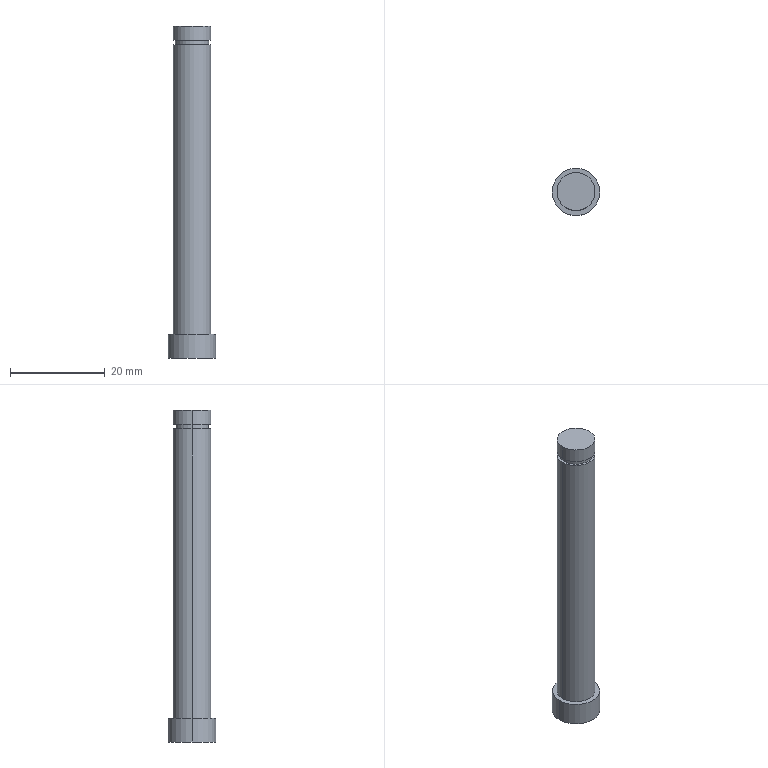Part | SolidWorks | features BaseBody 1 | 1 solid | 13 faces | box 10 x 10 x 70 mm | volume 3648 mm3 | cylinder 8 | plane 5 | commonest cylinder face diameters 8 x4 7 x2 10 x2
STEP:
#1=CARTESIAN_POINT('',(-4.,0.,67.));
#2=VERTEX_POINT('',#1);
#3=CARTESIAN_POINT('',(4.,0.,67.));
#4=VERTEX_POINT('',#3);
#5=CARTESIAN_POINT('',(0.,0.,67.));
#6=DIRECTION('',(0.,0.,-1.));
#7=DIRECTION('',(1.,0.,0.));
#8=AXIS2_PLACEMENT_3D('',#5,#6,#7);
#9=CIRCLE('',#8,4.);
#10=EDGE_CURVE('',#2,#4,#9,.T.);
#11=ORIENTED_EDGE('',*,*,#10,.F.);
#12=CARTESIAN_POINT('',(-4.,0.,70.));
#13=VERTEX_POINT('',#12);
#14=CARTESIAN_POINT('',(-4.,0.,5.));
#15=DIRECTION('',(0.,0.,1.));
#16=VECTOR('',#15,1000.);
#17=LINE('',#14,#16);
#18=EDGE_CURVE('',#2,#13,#17,.T.);
#19=ORIENTED_EDGE('',*,*,#18,.T.);
#20=CARTESIAN_POINT('',(4.,0.,70.));
#21=VERTEX_POINT('',#20);
#22=CARTESIAN_POINT('',(0.,0.,70.));
#23=DIRECTION('',(0.,0.,1.));
#24=DIRECTION('',(1.,0.,0.));
#25=AXIS2_PLACEMENT_3D('',#22,#23,#24);
#26=CIRCLE('',#25,4.);
#27=EDGE_CURVE('',#21,#13,#26,.T.);
#28=ORIENTED_EDGE('',*,*,#27,.F.);
#29=CARTESIAN_POINT('',(4.,0.,5.));
#30=DIRECTION('',(0.,0.,1.));
#31=VECTOR('',#30,1000.);
#32=LINE('',#29,#31);
#33=EDGE_CURVE('',#4,#21,#32,.T.);
#34=ORIENTED_EDGE('',*,*,#33,.F.);
#35=EDGE_LOOP('',(#11,#19,#28,#34));
#36=FACE_OUTER_BOUND('',#35,.T.);
#37=CARTESIAN_POINT('',(0.,0.,5.));
#38=DIRECTION('',(0.,0.,1.));
#39=DIRECTION('',(1.,0.,0.));
#40=AXIS2_PLACEMENT_3D('',#37,#38,#39);
#41=CYLINDRICAL_SURFACE('',#40,4.);
#42=ADVANCED_FACE('',(#36),#41,.T.);
#43=CARTESIAN_POINT('',(3.5,0.,66.));
#44=VERTEX_POINT('',#43);
#45=CARTESIAN_POINT('',(-3.5,0.,66.));
#46=VERTEX_POINT('',#45);
#47=CARTESIAN_POINT('',(0.,0.,66.));
#48=DIRECTION('',(0.,0.,1.));
#49=DIRECTION('',(1.,0.,0.));
#50=AXIS2_PLACEMENT_3D('',#47,#48,#49);
#51=CIRCLE('',#50,3.5);
#52=EDGE_CURVE('',#44,#46,#51,.T.);
#53=ORIENTED_EDGE('',*,*,#52,.T.);
#54=CARTESIAN_POINT('',(-3.5,0.,67.));
#55=VERTEX_POINT('',#54);
#56=CARTESIAN_POINT('',(-3.5,0.,66.));
#57=DIRECTION('',(0.,0.,1.));
#58=VECTOR('',#57,1000.);
#59=LINE('',#56,#58);
#60=EDGE_CURVE('',#46,#55,#59,.T.);
#61=ORIENTED_EDGE('',*,*,#60,.T.);
#62=CARTESIAN_POINT('',(3.5,0.,67.));
#63=VERTEX_POINT('',#62);
#64=CARTESIAN_POINT('',(0.,0.,67.));
#65=DIRECTION('',(0.,0.,1.));
#66=DIRECTION('',(1.,0.,0.));
#67=AXIS2_PLACEMENT_3D('',#64,#65,#66);
#68=CIRCLE('',#67,3.5);
#69=EDGE_CURVE('',#63,#55,#68,.T.);
#70=ORIENTED_EDGE('',*,*,#69,.F.);
#71=CARTESIAN_POINT('',(3.5,0.,66.));
#72=DIRECTION('',(0.,0.,1.));
#73=VECTOR('',#72,1000.);
#74=LINE('',#71,#73);
#75=EDGE_CURVE('',#44,#63,#74,.T.);
#76=ORIENTED_EDGE('',*,*,#75,.F.);
#77=EDGE_LOOP('',(#53,#61,#70,#76));
#78=FACE_OUTER_BOUND('',#77,.T.);
#79=CARTESIAN_POINT('',(0.,0.,66.));
#80=DIRECTION('',(0.,0.,1.));
#81=DIRECTION('',(1.,0.,0.));
#82=AXIS2_PLACEMENT_3D('',#79,#80,#81);
#83=CYLINDRICAL_SURFACE('',#82,3.5);
#84=ADVANCED_FACE('',(#78),#83,.T.);
#85=CARTESIAN_POINT('',(5.,0.,5.));
#86=VERTEX_POINT('',#85);
#87=CARTESIAN_POINT('',(-5.,0.,5.));
#88=VERTEX_POINT('',#87);
#89=CARTESIAN_POINT('',(0.,0.,5.));
#90=DIRECTION('',(0.,0.,1.));
#91=DIRECTION('',(1.,0.,0.));
#92=AXIS2_PLACEMENT_3D('',#89,#90,#91);
#93=CIRCLE('',#92,5.);
#94=EDGE_CURVE('',#86,#88,#93,.T.);
#95=ORIENTED_EDGE('',*,*,#94,.F.);
#96=CARTESIAN_POINT('',(5.,0.,0.));
#97=VERTEX_POINT('',#96);
#98=CARTESIAN_POINT('',(5.,0.,70.));
#99=DIRECTION('',(0.,0.,-1.));
#100=VECTOR('',#99,1000.);
#101=LINE('',#98,#100);
#102=EDGE_CURVE('',#86,#97,#101,.T.);
#103=ORIENTED_EDGE('',*,*,#102,.T.);
#104=CARTESIAN_POINT('',(-5.,0.,0.));
#105=VERTEX_POINT('',#104);
#106=CARTESIAN_POINT('',(0.,0.,0.));
#107=DIRECTION('',(0.,0.,1.));
#108=DIRECTION('',(1.,0.,0.));
#109=AXIS2_PLACEMENT_3D('',#106,#107,#108);
#110=CIRCLE('',#109,5.);
#111=EDGE_CURVE('',#97,#105,#110,.T.);
#112=ORIENTED_EDGE('',*,*,#111,.T.);
#113=CARTESIAN_POINT('',(-5.,0.,70.));
#114=DIRECTION('',(0.,0.,-1.));
#115=VECTOR('',#114,1000.);
#116=LINE('',#113,#115);
#117=EDGE_CURVE('',#88,#105,#116,.T.);
#118=ORIENTED_EDGE('',*,*,#117,.F.);
#119=EDGE_LOOP('',(#95,#103,#112,#118));
#120=FACE_OUTER_BOUND('',#119,.T.);
#121=CARTESIAN_POINT('',(0.,0.,70.));
#122=DIRECTION('',(0.,0.,-1.));
#123=DIRECTION('',(-1.,0.,0.));
#124=AXIS2_PLACEMENT_3D('',#121,#122,#123);
#125=CYLINDRICAL_SURFACE('',#124,5.);
#126=ADVANCED_FACE('',(#120),#125,.T.);
#127=CARTESIAN_POINT('',(4.,0.,5.));
#128=VERTEX_POINT('',#127);
#129=CARTESIAN_POINT('',(-4.,0.,5.));
#130=VERTEX_POINT('',#129);
#131=CARTESIAN_POINT('',(0.,0.,5.));
#132=DIRECTION('',(0.,0.,1.));
#133=DIRECTION('',(1.,0.,0.));
#134=AXIS2_PLACEMENT_3D('',#131,#132,#133);
#135=CIRCLE('',#134,4.);
#136=EDGE_CURVE('',#128,#130,#135,.T.);
#137=ORIENTED_EDGE('',*,*,#136,.T.);
#138=CARTESIAN_POINT('',(-4.,0.,66.));
#139=VERTEX_POINT('',#138);
#140=CARTESIAN_POINT('',(-4.,0.,5.));
#141=DIRECTION('',(0.,0.,1.));
#142=VECTOR('',#141,1000.);
#143=LINE('',#140,#142);
#144=EDGE_CURVE('',#130,#139,#143,.T.);
#145=ORIENTED_EDGE('',*,*,#144,.T.);
#146=CARTESIAN_POINT('',(4.,0.,66.));
#147=VERTEX_POINT('',#146);
#148=CARTESIAN_POINT('',(0.,0.,66.));
#149=DIRECTION('',(0.,0.,-1.));
#150=DIRECTION('',(1.,0.,0.));
#151=AXIS2_PLACEMENT_3D('',#148,#149,#150);
#152=CIRCLE('',#151,4.);
#153=EDGE_CURVE('',#139,#147,#152,.T.);
#154=ORIENTED_EDGE('',*,*,#153,.T.);
#155=CARTESIAN_POINT('',(4.,0.,5.));
#156=DIRECTION('',(0.,0.,1.));
#157=VECTOR('',#156,1000.);
#158=LINE('',#155,#157);
#159=EDGE_CURVE('',#128,#147,#158,.T.);
#160=ORIENTED_EDGE('',*,*,#159,.F.);
#161=EDGE_LOOP('',(#137,#145,#154,#160));
#162=FACE_OUTER_BOUND('',#161,.T.);
#163=CARTESIAN_POINT('',(0.,0.,5.));
#164=DIRECTION('',(0.,0.,1.));
#165=DIRECTION('',(1.,0.,0.));
#166=AXIS2_PLACEMENT_3D('',#163,#164,#165);
#167=CYLINDRICAL_SURFACE('',#166,4.);
#168=ADVANCED_FACE('',(#162),#167,.T.);
#169=ORIENTED_EDGE('',*,*,#27,.T.);
#170=CARTESIAN_POINT('',(0.,0.,70.));
#171=DIRECTION('',(0.,0.,1.));
#172=DIRECTION('',(1.,0.,0.));
#173=AXIS2_PLACEMENT_3D('',#170,#171,#172);
#174=CIRCLE('',#173,4.);
#175=EDGE_CURVE('',#13,#21,#174,.T.);
#176=ORIENTED_EDGE('',*,*,#175,.T.);
#177=EDGE_LOOP('',(#169,#176));
#178=FACE_OUTER_BOUND('',#177,.T.);
#179=CARTESIAN_POINT('',(0.,0.,70.));
#180=DIRECTION('',(0.,0.,1.));
#181=DIRECTION('',(1.,0.,0.));
#182=AXIS2_PLACEMENT_3D('',#179,#180,#181);
#183=PLANE('',#182);
#184=ADVANCED_FACE('',(#178),#183,.T.);
#185=ORIENTED_EDGE('',*,*,#69,.T.);
#186=CARTESIAN_POINT('',(0.,0.,67.));
#187=DIRECTION('',(0.,0.,1.));
#188=DIRECTION('',(1.,0.,0.));
#189=AXIS2_PLACEMENT_3D('',#186,#187,#188);
#190=CIRCLE('',#189,3.5);
#191=EDGE_CURVE('',#55,#63,#190,.T.);
#192=ORIENTED_EDGE('',*,*,#191,.T.);
#193=EDGE_LOOP('',(#185,#192));
#194=FACE_BOUND('',#193,.T.);
#195=CARTESIAN_POINT('',(0.,0.,67.));
#196=DIRECTION('',(0.,0.,-1.));
#197=DIRECTION('',(1.,0.,0.));
#198=AXIS2_PLACEMENT_3D('',#195,#196,#197);
#199=CIRCLE('',#198,4.);
#200=EDGE_CURVE('',#4,#2,#199,.T.);
#201=ORIENTED_EDGE('',*,*,#200,.T.);
#202=ORIENTED_EDGE('',*,*,#10,.T.);
#203=EDGE_LOOP('',(#201,#202));
#204=FACE_OUTER_BOUND('',#203,.T.);
#205=CARTESIAN_POINT('',(0.,0.,67.));
#206=DIRECTION('',(0.,0.,1.));
#207=DIRECTION('',(1.,0.,0.));
#208=AXIS2_PLACEMENT_3D('',#205,#206,#207);
#209=PLANE('',#208);
#210=ADVANCED_FACE('',(#194,#204),#209,.F.);
#211=ORIENTED_EDGE('',*,*,#52,.F.);
#212=CARTESIAN_POINT('',(0.,0.,66.));
#213=DIRECTION('',(0.,0.,1.));
#214=DIRECTION('',(1.,0.,0.));
#215=AXIS2_PLACEMENT_3D('',#212,#213,#214);
#216=CIRCLE('',#215,3.5);
#217=EDGE_CURVE('',#46,#44,#216,.T.);
#218=ORIENTED_EDGE('',*,*,#217,.F.);
#219=EDGE_LOOP('',(#211,#218));
#220=FACE_BOUND('',#219,.T.);
#221=CARTESIAN_POINT('',(0.,0.,66.));
#222=DIRECTION('',(0.,0.,-1.));
#223=DIRECTION('',(1.,0.,0.));
#224=AXIS2_PLACEMENT_3D('',#221,#222,#223);
#225=CIRCLE('',#224,4.);
#226=EDGE_CURVE('',#147,#139,#225,.T.);
#227=ORIENTED_EDGE('',*,*,#226,.F.);
#228=ORIENTED_EDGE('',*,*,#153,.F.);
#229=EDGE_LOOP('',(#227,#228));
#230=FACE_OUTER_BOUND('',#229,.T.);
#231=CARTESIAN_POINT('',(0.,0.,66.));
#232=DIRECTION('',(0.,0.,1.));
#233=DIRECTION('',(1.,0.,0.));
#234=AXIS2_PLACEMENT_3D('',#231,#232,#233);
#235=PLANE('',#234);
#236=ADVANCED_FACE('',(#220,#230),#235,.T.);
#237=ORIENTED_EDGE('',*,*,#136,.F.);
#238=CARTESIAN_POINT('',(0.,0.,5.));
#239=DIRECTION('',(0.,0.,1.));
#240=DIRECTION('',(1.,0.,0.));
#241=AXIS2_PLACEMENT_3D('',#238,#239,#240);
#242=CIRCLE('',#241,4.);
#243=EDGE_CURVE('',#130,#128,#242,.T.);
#244=ORIENTED_EDGE('',*,*,#243,.F.);
#245=EDGE_LOOP('',(#237,#244));
#246=FACE_BOUND('',#245,.T.);
#247=CARTESIAN_POINT('',(0.,0.,5.));
#248=DIRECTION('',(0.,0.,1.));
#249=DIRECTION('',(1.,0.,0.));
#250=AXIS2_PLACEMENT_3D('',#247,#248,#249);
#251=CIRCLE('',#250,5.);
#252=EDGE_CURVE('',#88,#86,#251,.T.);
#253=ORIENTED_EDGE('',*,*,#252,.T.);
#254=ORIENTED_EDGE('',*,*,#94,.T.);
#255=EDGE_LOOP('',(#253,#254));
#256=FACE_OUTER_BOUND('',#255,.T.);
#257=CARTESIAN_POINT('',(0.,0.,5.));
#258=DIRECTION('',(0.,0.,1.));
#259=DIRECTION('',(1.,0.,0.));
#260=AXIS2_PLACEMENT_3D('',#257,#258,#259);
#261=PLANE('',#260);
#262=ADVANCED_FACE('',(#246,#256),#261,.T.);
#263=CARTESIAN_POINT('',(0.,0.,0.));
#264=DIRECTION('',(0.,0.,1.));
#265=DIRECTION('',(1.,0.,0.));
#266=AXIS2_PLACEMENT_3D('',#263,#264,#265);
#267=CIRCLE('',#266,5.);
#268=EDGE_CURVE('',#105,#97,#267,.T.);
#269=ORIENTED_EDGE('',*,*,#268,.F.);
#270=ORIENTED_EDGE('',*,*,#111,.F.);
#271=EDGE_LOOP('',(#269,#270));
#272=FACE_OUTER_BOUND('',#271,.T.);
#273=CARTESIAN_POINT('',(0.,0.,0.));
#274=DIRECTION('',(0.,0.,1.));
#275=DIRECTION('',(1.,0.,0.));
#276=AXIS2_PLACEMENT_3D('',#273,#274,#275);
#277=PLANE('',#276);
#278=ADVANCED_FACE('',(#272),#277,.F.);
#279=ORIENTED_EDGE('',*,*,#144,.F.);
#280=ORIENTED_EDGE('',*,*,#243,.T.);
#281=ORIENTED_EDGE('',*,*,#159,.T.);
#282=ORIENTED_EDGE('',*,*,#226,.T.);
#283=EDGE_LOOP('',(#279,#280,#281,#282));
#284=FACE_OUTER_BOUND('',#283,.T.);
#285=CARTESIAN_POINT('',(0.,0.,5.));
#286=DIRECTION('',(0.,0.,1.));
#287=DIRECTION('',(1.,0.,0.));
#288=AXIS2_PLACEMENT_3D('',#285,#286,#287);
#289=CYLINDRICAL_SURFACE('',#288,4.);
#290=ADVANCED_FACE('',(#284),#289,.T.);
#291=ORIENTED_EDGE('',*,*,#102,.F.);
#292=ORIENTED_EDGE('',*,*,#252,.F.);
#293=ORIENTED_EDGE('',*,*,#117,.T.);
#294=ORIENTED_EDGE('',*,*,#268,.T.);
#295=EDGE_LOOP('',(#291,#292,#293,#294));
#296=FACE_OUTER_BOUND('',#295,.T.);
#297=CARTESIAN_POINT('',(0.,0.,70.));
#298=DIRECTION('',(0.,0.,-1.));
#299=DIRECTION('',(-1.,0.,0.));
#300=AXIS2_PLACEMENT_3D('',#297,#298,#299);
#301=CYLINDRICAL_SURFACE('',#300,5.);
#302=ADVANCED_FACE('',(#296),#301,.T.);
#303=ORIENTED_EDGE('',*,*,#60,.F.);
#304=ORIENTED_EDGE('',*,*,#217,.T.);
#305=ORIENTED_EDGE('',*,*,#75,.T.);
#306=ORIENTED_EDGE('',*,*,#191,.F.);
#307=EDGE_LOOP('',(#303,#304,#305,#306));
#308=FACE_OUTER_BOUND('',#307,.T.);
#309=CARTESIAN_POINT('',(0.,0.,66.));
#310=DIRECTION('',(0.,0.,1.));
#311=DIRECTION('',(1.,0.,0.));
#312=AXIS2_PLACEMENT_3D('',#309,#310,#311);
#313=CYLINDRICAL_SURFACE('',#312,3.5);
#314=ADVANCED_FACE('',(#308),#313,.T.);
#315=ORIENTED_EDGE('',*,*,#18,.F.);
#316=ORIENTED_EDGE('',*,*,#200,.F.);
#317=ORIENTED_EDGE('',*,*,#33,.T.);
#318=ORIENTED_EDGE('',*,*,#175,.F.);
#319=EDGE_LOOP('',(#315,#316,#317,#318));
#320=FACE_OUTER_BOUND('',#319,.T.);
#321=CARTESIAN_POINT('',(0.,0.,5.));
#322=DIRECTION('',(0.,0.,1.));
#323=DIRECTION('',(1.,0.,0.));
#324=AXIS2_PLACEMENT_3D('',#321,#322,#323);
#325=CYLINDRICAL_SURFACE('',#324,4.);
#326=ADVANCED_FACE('',(#320),#325,.T.);
#327=CLOSED_SHELL('',(#42,#84,#126,#168,#184,#210,#236,#262,#278,#290,#302,#314,#326));
#328=MANIFOLD_SOLID_BREP('',#327);
#329=CARTESIAN_POINT('',(0.,0.,0.));
#330=DIRECTION('',(0.,0.,1.));
#331=DIRECTION('',(1.,0.,0.));
#332=AXIS2_PLACEMENT_3D('',#329,#330,#331);
#333=(LENGTH_UNIT()NAMED_UNIT(*)SI_UNIT(.MILLI.,.METRE.));
#334=UNCERTAINTY_MEASURE_WITH_UNIT(LENGTH_MEASURE(0.00001),#333,'','');
#335=(NAMED_UNIT(*)PLANE_ANGLE_UNIT()SI_UNIT($,.RADIAN.));
#336=(NAMED_UNIT(*)SI_UNIT($,.STERADIAN.)SOLID_ANGLE_UNIT());
#337=(GEOMETRIC_REPRESENTATION_CONTEXT(3)GLOBAL_UNCERTAINTY_ASSIGNED_CONTEXT((#334))GLOBAL_UNIT_ASSIGNED_CONTEXT((#333,#335,#336))REPRESENTATION_CONTEXT('',''));
#338=ADVANCED_BREP_SHAPE_REPRESENTATION('',(#328,#332),#337);